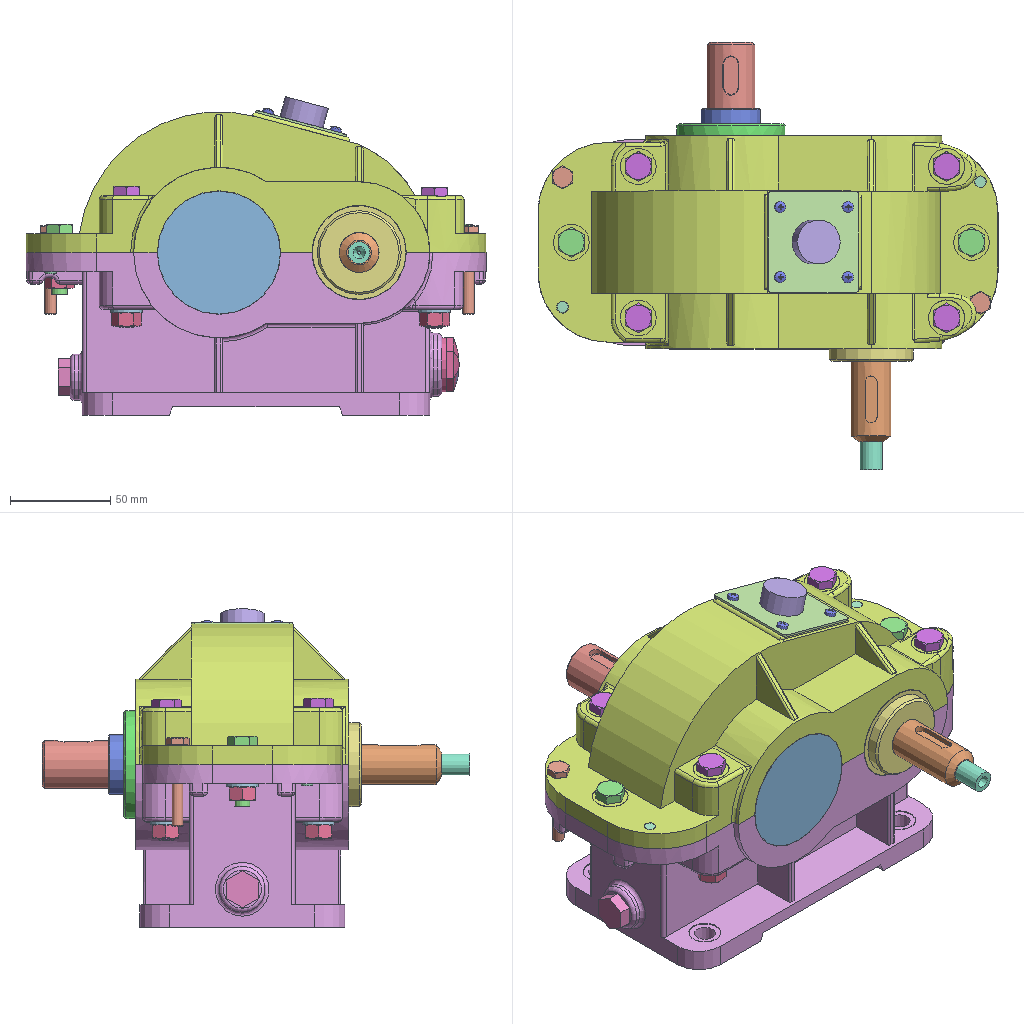Assembly | NX | 31 different items | 52 placed | box 230 x 213 x 159 mm
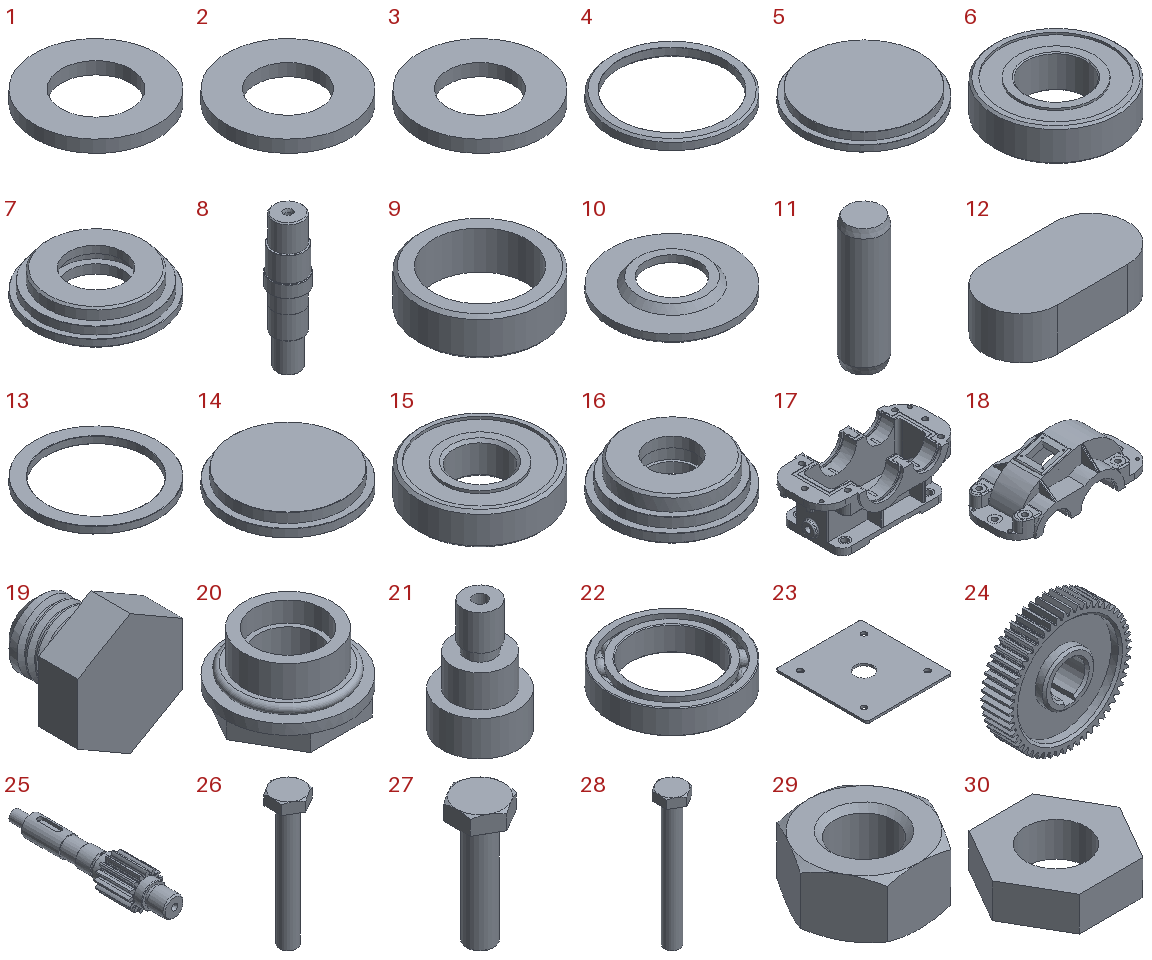Parts list (item | quantity | size | volume | features):
1 | x5 | 16 x 16 x 1.6 mm | 219.911 mm3 | features DATUM_CSYS 2, LINE 1, SKETCH 1, SWP104 1
2 | x1 | 20 x 20 x 2 mm | 455.138 mm3 | features DATUM_CSYS 2, EXTRUDE 1, LINE 1, SKETCH 1
3 | x1 | 16 x 16 x 1.6 mm | 233.031 mm3 | features DATUM_CSYS 2, EXTRUDE 1, LINE 1, SKETCH 1
4 | x1 | 61.62 x 61.62 x 4.68 mm | 3737 mm3 | features CHAMFER 4, DATUM_CSYS 2, EXTRUDE 1, SKETCH 1
5 | x1 | 67.2 x 67.2 x 7.62 mm | 18147 mm3 | features CHAMFER 4, DATUM_CSYS 4, EXTRUDE 3, SKETCH 3, DATUM_PLANE 1
6 | x2 | 61.62 x 61.62 x 16.4 mm | 34698 mm3 | features CHAMFER 4, DATUM_CSYS 4, EXTRUDE 3, SKETCH 3, DATUM_PLANE 2
7 | x1 | 67.2 x 67.2 x 16.58 mm | 29560 mm3 | features DATUM_CSYS 9, SKETCH 8, EXTRUDE 7, CHAMFER 6, DATUM_PLANE 3, Resize Face 2
8 | x1 | 36 x 36 x 139.56 mm | 97541 mm3 | features CHAMFER 9, CYLINDER 6, DATUM_CSYS 3, DATUM_PLANE 2, EXTRUDE 2, SKETCH 2, U_SLOT 2, RECT_GROOVE 1, Resize Face 1
9 | x1 | 39.74 x 39.74 x 12.34 mm | 6461 mm3 | features CHAMFER 2, DATUM_CSYS 2, EXTRUDE 1, SKETCH 1
10 | x2 | 47.08 x 47.08 x 6 mm | 4835 mm3 | features DATUM_CSYS 2, CHAMFER 1, SKETCH 1, SWP104 1
11 | x2 | 6 x 6 x 20 mm | 558.473 mm3 | features DATUM_CSYS 2, LINE 1, SKETCH 1, SWP104 1
12 | x1 | 19.6 x 10 x 5.8 mm | 1012 mm3 | features DATUM_CSYS 2, EXTRUDE 1, SKETCH 1
13 | x1 | 47.08 x 47.08 x 2.66 mm | 1678 mm3 | features CHAMFER 3, DATUM_CSYS 2, EXTRUDE 1, SKETCH 1
14 | x1 | 52.42 x 52.42 x 7.62 mm | 11135 mm3 | features CHAMFER 4, DATUM_CSYS 4, EXTRUDE 3, SKETCH 3, DATUM_PLANE 2
15 | x2 | 47.08 x 47.08 x 12.42 mm | 15931 mm3 | features CHAMFER 4, DATUM_CSYS 4, EXTRUDE 3, SKETCH 3, DATUM_PLANE 1
16 | x1 | 52.42 x 52.42 x 15.88 mm | 19851 mm3 | features CHAMFER 8, DATUM_CSYS 8, SKETCH 7, EXTRUDE 6, DATUM_PLANE 5, DISTANCE MEASUREMENT 2, Resize Face 2
17 | x1 | 229.56 x 106.4 x 81.2 mm | 501453 mm3 | features EXTRUDE 28, BLEND 23, DATUM_CSYS 21, SKETCH 20, EXTRACT_STRING 8, Instance Feature 4, MIRROR_CURVE 4, Mirror Feature 4, DATUM_PLANE 3, FACE_BLEND 3, RIB 3, CPROJ 2, REPLACE_FACE 2, U_SLOT 2, SYMBOLIC_THREAD 1
18 | x1 | 229.56 x 106.4 x 70.29 mm | 339621 mm3 | features DATUM_CSYS 18, EXTRUDE 18, SKETCH 17, BLEND 13, EXTRACT_STRING 6, SYMBOLIC_THREAD 6, Instance Feature 4, Mirror Feature 4, RIB 4, ASSOCIATIVE_INTERSECTION 2, CHAMFER 2, DATUM_PLANE 2, EXTRACT_FACE 2, REPLACE_FACE 2
19 | x1 | 16 x 15 x 18.475 mm | 1967 mm3 | features DATUM_CSYS 3, SKETCH 2, EXTRUDE 1, SWP104 1, THREADS 1
20 | x1 | 27 x 27 x 17.442 mm | 4366 mm3 | features DATUM_CSYS 8, SKETCH 7, EXTRUDE 6, EXTRACT_BODY 5, EXTRACT_STRING 5, BLEND 2, Pattern Geometry 2, UNITE 2, FILL_HOLE 1, SYMBOLIC_THREAD 1, THICKEN_SHEET 1
21 | x1 | 22.2 x 22.2 x 32.8 mm | 6457 mm3 | features DATUM_CSYS 5, CYLINDER 4, EXTRUDE 4, SKETCH 4, DATUM_PLANE 1, SYMBOLIC_THREAD 1
22 | x1 | 15 x 15 x 3 mm | 196.013 mm3 | features SWP104 18, INSTANCE_SET 13, SKETCH 4, CHAMFER 2, DATUM_CSYS 2, FSET 2, CIRCULAR_PATTERN 1, LINE 1
23 | x1 | 47 x 50.372 x 1.2 mm | 2711 mm3 | features DATUM_CSYS 2, EXTRUDE 1, SKETCH 1
24 | x1 | 113.946 x 26 x 113.987 mm | 134630 mm3 | features BREP 55, META 55, DATUM_CSYS 4, EXTRUDE 3, SKETCH 3, EXTRACT_DATUM_AXIS 2, EXTRACT_DATUM_PLANE 2, EXTRACT_STRING 2, CHAMFER 1, CYLINDER 1, FSET 1, Instance Feature 1, Mirror Feature 1
25 | x1 | 33.753 x 158.547 x 33.926 mm | 59659 mm3 | features BREP 15, META 15, DATUM_CSYS 11, SKETCH 10, EXTRUDE 8, CHAMFER 4, DATUM_PLANE 2, HOLE PACKAGE 2, TAPER_HOLE 2, CYLINDER 1, FSET 1, RECT_SLOT 1, Resize Face 1, SWP104 1, SYMBOLIC_THREAD 1
26 | x2 | 10 x 11.547 x 44 mm | 1387 mm3 | features SKETCH 4, EXTRUDE 3, META 3, DATUM_CSYS 2, BLEND 1, CHAMFER 1, LINE 1, SWP104 1, SYMBOLIC_THREAD 1, THREADS 1
27 | x2 | 13 x 15.011 x 35.3 mm | 2165 mm3 | features SKETCH 4, EXTRUDE 3, META 3, DATUM_CSYS 2, BLEND 1, CHAMFER 1, LINE 1, SWP104 1, SYMBOLIC_THREAD 1, THREADS 1
28 | x4 | 13 x 15.011 x 70.3 mm | 3821 mm3 | features SKETCH 4, EXTRUDE 3, META 3, DATUM_CSYS 2, BLEND 1, CHAMFER 1, LINE 1, SWP104 1, SYMBOLIC_THREAD 1, THREADS 1
29 | x6 | 15.011 x 13 x 6.8 mm | 719.574 mm3 | features META 3, SKETCH 3, DATUM_CSYS 2, EXTRUDE 2, SWP104 2, CHAMFER 1, LINE 1, SYMBOLIC_THREAD 1, THREADS 1
30 | x1 | 18.475 x 16 x 5 mm | 805.635 mm3 | features SKETCH 3, DATUM_CSYS 2, EXTRUDE 2, LINE 1, META 1, SYMBOLIC_THREAD 1, THREADS 1
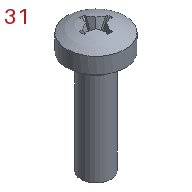31 | x4 | 5.6 x 5.6 x 12.351 mm | 111.736 mm3 | features SKETCH 3, DATUM_CSYS 2, DATUM_PLANE 2, FSET 1, LINE 1, META 1, SKIN 1, SWP104 1, SYMBOLIC_THREAD 1, THREADS 1
Mates (type | each side: item.copy, entity, surface, feature):
Fix | 17.1 component
Touch | 18.1 face cylinder Extrude(43) | 17.1 face cylinder Extrude(91)
Touch | 18.1 face plane Extrude(2) | 17.1 face plane Extrude(6)
Touch | 5.1 face cylinder Extrude(7) | 17.1 face cylinder Extrude(10)
Touch | 5.1 face plane Extrude(7) | 17.1 face plane Extrude(32)
Touch | 17.1 face cylinder Extrude(10) | 4.1 face cylinder Extrude(2)
Touch | 4.1 face plane Extrude(2) | 5.1 face plane Extrude(2)
Touch | 7.1 face cylinder Extrude(14) | 17.1 face cylinder Extrude(10)
Touch | 7.1 face plane Extrude(16) | 17.1 face plane Mirror Feature(33)
Touch | 6.1 face cylinder Extrude(2) | 7.1 face cylinder Extrude(5)
Touch | 6.1 face plane Extrude(2) | 7.1 face plane Extrude(2)
Touch | 8.1 face cylinder Cylinder(1) | 17.1 face cylinder Extrude(10)
Distance | 8.1 face plane Cylinder(1) | 17.1 face plane Extrude(10)
Touch | 9.1 face cylinder Extrude(2) | 8.1 face cylinder Cylinder(2)
Touch | 9.1 face plane Extrude(2) | 8.1 face plane Cylinder(2)
Touch | 14.1 face cylinder Extrude(6) | 17.1 face cylinder Extrude(10)
Touch | 14.1 face plane Extrude(3) | 17.1 face plane Mirror Feature(11)
Touch | 16.1 face cylinder Extrude(2) | 17.1 face cylinder Extrude(10)
Touch | 16.1 face plane Extrude(17) | 17.1 face plane Extrude(32)
Touch | 13.1 face cylinder Extrude(2) | 14.1 face cylinder Extrude(3)
Touch | 13.1 face plane Extrude(2) | 14.1 face plane Extrude(3)
Touch | 20.1 face cylinder Extrude(11) | 17.1 face cylinder Extrude(83)
Touch | 20.1 face plane Extrude(2) | 17.1 face plane Extrude(83)
Touch | 10.1 face cone Revolve(2) | 13.1 face cylinder Extrude(2)
Touch | 25.1 face cylinder Extrude(40) | 17.1 face cylinder Extrude(10)
Distance | 25.1 face plane Extrude(35) | 17.1 face plane Mirror Feature(11)
Touch | 10.1 face plane Revolve(2) | 17.1 face plane Extrude(23)
Touch | 15.1 face cylinder Extrude(2) | 25.1 face cylinder Extrude(35)
Touch | 15.1 face plane Extrude(2) | 10.1 face plane Revolve(2)
Touch | 19.1 face cylinder Revolve(4) | 17.1 face cylinder Extrude(86)
Touch | 19.1 face plane Extrude(2) | 17.1 face plane Extrude(86)
Parallel | 23.1 face plane Extrude(2) | 18.1 face plane Extrude(38)
Touch | 23.1 face cylinder Extrude(2) | 18.1 face cylinder Extrude(41)
Touch | 23.1 face plane Extrude(2) | 18.1 face plane Extrude(38)
Touch | 31.1 face cylinder Revolve(5) | 18.1 face cylinder Extrude(41)
Touch | 31.1 face plane Revolve(5) | 23.1 face plane Extrude(2) | 2 times
Touch | 31.1 face cylinder Revolve(5) | 23.1 face cylinder Extrude(2)
Touch | 26.1 face cylinder Extrude(9) | 18.1 face cylinder Extrude(45) | 2 times
Touch | 26.1 face plane Extrude(7) | 18.1 face plane Extrude(2) | 2 times
Touch | 11.1 face cylinder Revolve(16) | 18.1 face cylinder Extrude(46) | 2 times
Touch | 11.1 face plane Revolve(16) | 18.1 face plane Extrude(2) | 2 times
Touch | 28.1 face cylinder Extrude(9) | 18.1 face cylinder Extrude(43) | 2 times
Touch | 28.1 face plane Extrude(6) | 18.1 face plane Extrude(26) | 2 times
Touch | 1.1 face cylinder Revolve(16) | 17.1 face cylinder Extrude(43) | 2 times
Touch | 1.1 face plane Revolve(16) | 17.1 face plane Extrude(16)
Touch | 3.1 face cylinder Extrude(16) | 17.1 face cylinder Extrude(91)
Touch | 3.1 face plane Extrude(16) | 17.1 face plane Extrude(8)
Touch | 1.1 edge | 17.1 face plane Extrude(13)
Touch | 28.1 edge | 18.1 face plane Extrude(26)
Touch | 27.1 face cylinder Extrude(9) | 18.1 face cylinder Extrude(43)
Touch | 27.1 face plane Extrude(7) | 18.1 face plane Extrude(28)
Touch | 21.1 face cylinder Cylinder(4) | 23.1 face cylinder Extrude(2)
Touch | 21.1 face plane Cylinder(1) | 23.1 face plane Extrude(2)
Touch | 24.1 face cylinder Extrude(119) | 8.1 face cylinder Cylinder(6)
Touch | 24.1 face plane Cylinder(1) | 9.1 face plane Extrude(2)